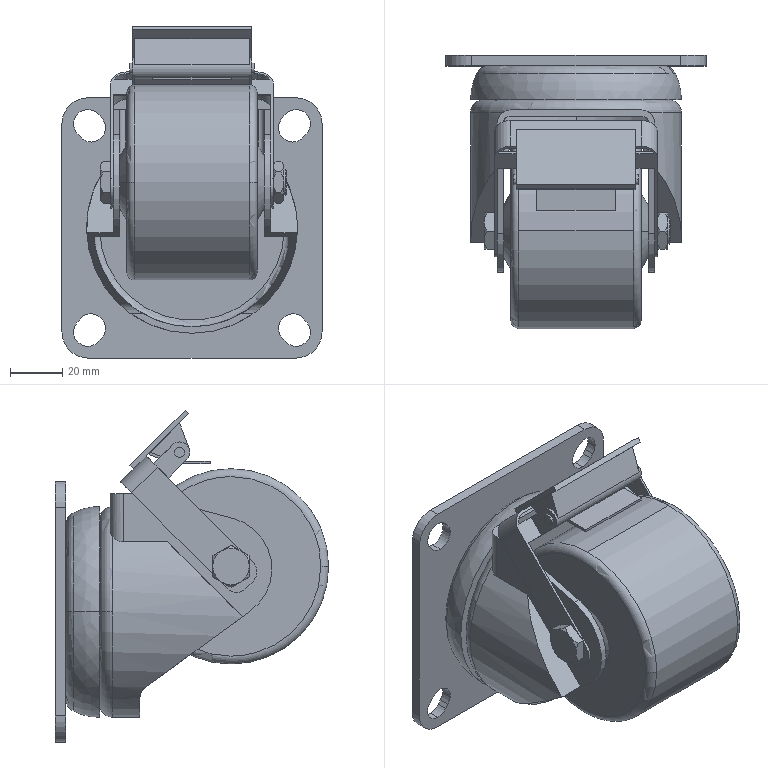Part | SolidWorks | features BaseBody 4 | 4 solids | 238 faces | box 100 x 105 x 127.604 mm | volume 370693 mm3 | plane 132 | cylinder 59 | cone 27 | torus 10 | spline 10 | commonest cylinder face diameters 10 x22 11 x12 4 x6 8 x5 20 x4 12 x3